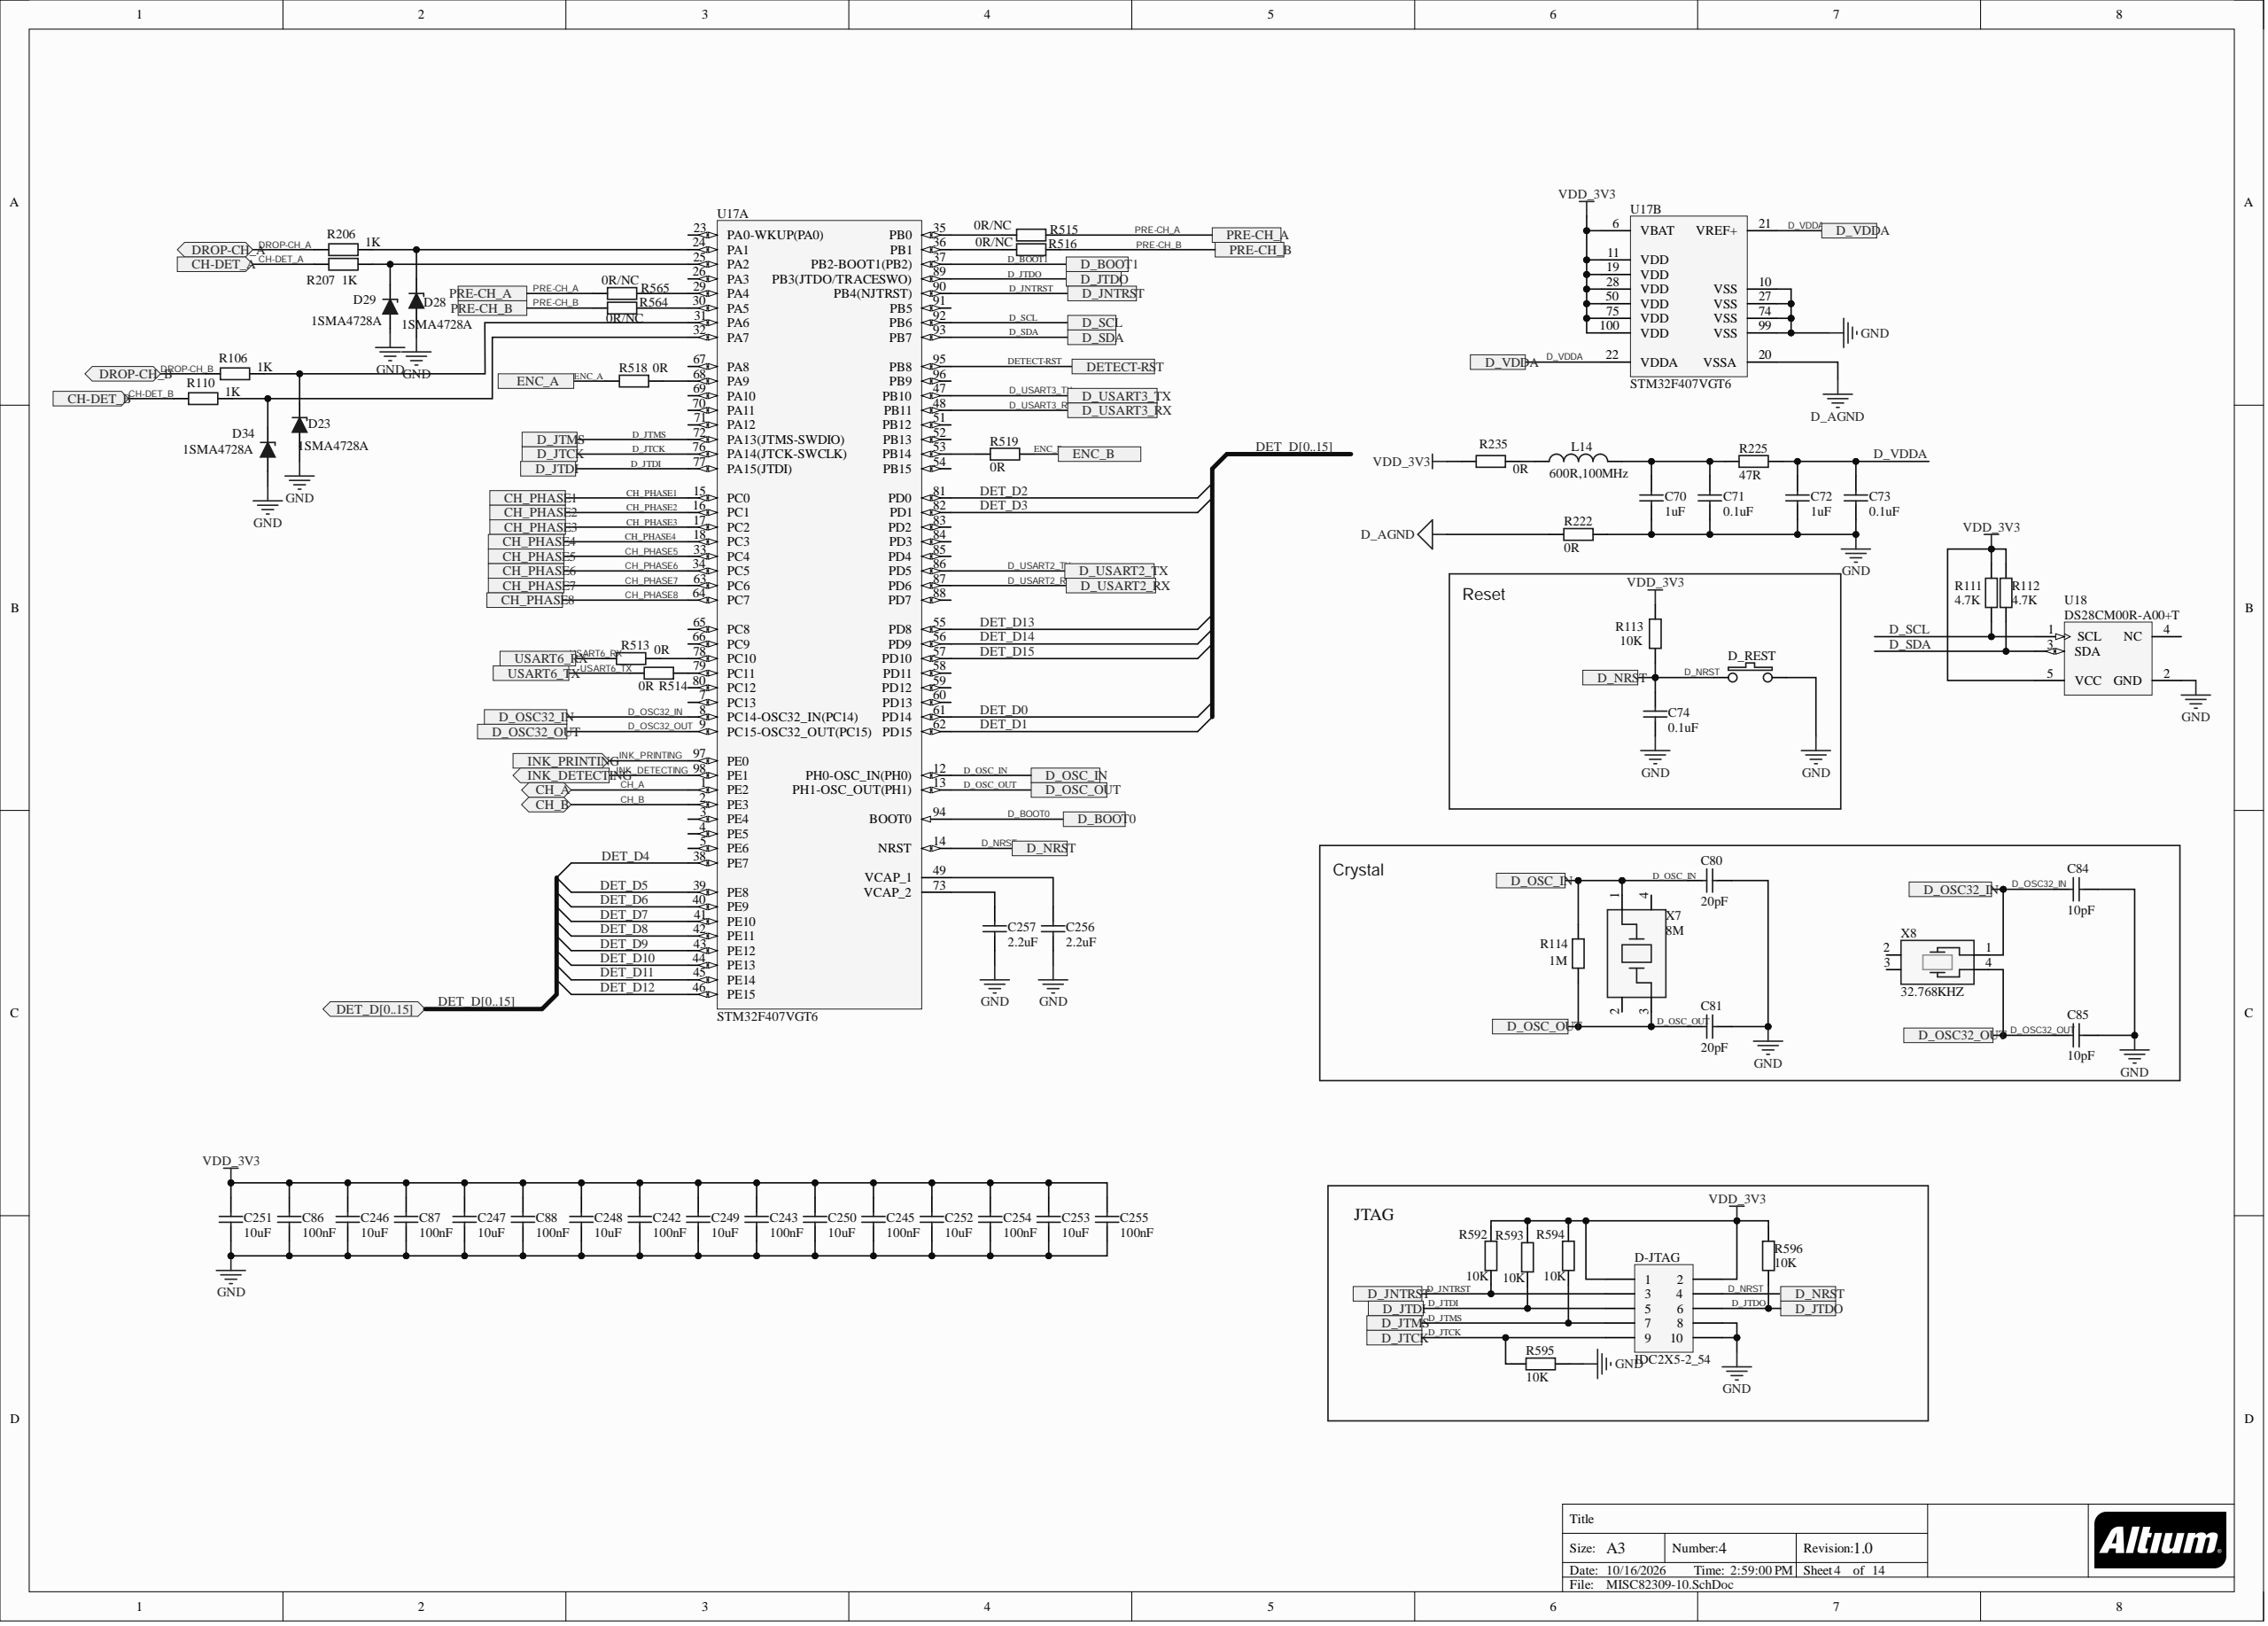Circuit board | Altium Designer | 747 parts | 576 nets | one sheet of the schematic
Parts on this sheet (reference | value | footprint):
C70 | 1uF | CAP_0805
C71 | 0.1uF | CAP_0805
C72 | 1uF | CAP_0805
C73 | 0.1uF | CAP_0805
C74 | 0.1uF | C0603
C80 | 20pF | C0603
C81 | 20pF | C0603
C84 | 10pF | C0603
C85 | 10pF | C0603
C86 | 100nF | C0805
C87 | 100nF | C0805
C88 | 100nF | C0805
C242 | 100nF | C0805
C243 | 100nF | C0805
C245 | 100nF | C0805
C246 | 10uF | C0805
C247 | 10uF | C0805
C248 | 10uF | C0805
C249 | 10uF | C0805
C250 | 10uF | C0805
C251 | 10uF | C0805
C252 | 10uF | C0805
C253 | 10uF | C0805
C254 | 100nF | C0805
C255 | 100nF | C0805
C256 | 2.2uF | CAP_0805
C257 | 2.2uF | CAP_0805
D23 | 1SMA4728A | DO-214AC
D28 | 1SMA4728A | DO-214AC
D29 | 1SMA4728A | DO-214AC
D34 | 1SMA4728A | DO-214AC
D-JTAG | IDC2X5-2_54 | IDC2X5-2_54
D_REST | SW | SW-6X3X2.5
L14 | 600R,100MHz | R0805
R106 | 1K | R1206
R110 | 1K | R1206
R111 | 4.7K | R0603
R112 | 4.7K | R0603
R113 | 10K | R0603
R114 | 1M | R0603
R206 | 1K | R1206
R207 | 1K | R1206
R222 | 0R | R0805
R225 | 47R | R0805
R235 | 0R | R0805
R513 | 0R | RES_0603
R514 | 0R | RES_0603
R515 | 0R/NC | RES_0603
R516 | 0R/NC | RES_0603
R518 | 0R | RES_0603
R519 | 0R | RES_0603
R564 | 0R/NC | RES_0603
R565 | 0R/NC | RES_0603
R592 | 10K | R0603
R593 | 10K | R0603
R594 | 10K | R0603
R595 | 10K | R0603
R596 | 10K | R0603
U17 | STM32F407VGT6 | LQFP100_N
U18 | DS28CM00R-A00+T | U5+1_N
X7 | 8M | SMD5032
X8 | 32.768KHz | Y_XTAL_T7
Nets of these parts (net: part-pin ...):
VDD_3V3: C86-2 C87-2 C88-2 C242-2 C243-2 C245-2 C246-2 C247-2 C248-2 C249-2 C250-2 C251-2 C252-2 C253-2 C254-2 C255-2 D-JTAG-1 D-JTAG-2 R111-1 R112-1 R113-1 R235-1 R592-2 R593-2 R594-2 R596-1 U18-5 U17-6 U17-11 U17-19 U17-28 U17-50 U17-75 U17-100
USART6_TX: R514-2
USART6_RX: R513-2
PRE-CH_B: R516-2 R564-1
PRE-CH_A: R515-2 R565-1
NetR565_2: R565-2 U17-29
NetR564_2: R564-2 U17-30
NetR519_1: R519-1 U17-53
NetR518_1: R518-1 U17-68
NetR516_1: R516-1 U17-36
NetR515_1: R515-1 U17-35
NetR514_1: R514-1 U17-79
NetR513_1: R513-1 U17-78
NetL14_1: L14-1 R235-2
NetD34_2: D34-2 R110-2 U17-32
NetD29_2: D29-2 R207-2 U17-25
NetD28_2: D28-2 R206-2 U17-24
NetD23_2: D23-2 R106-2 U17-31
NetC257_1: C257-1 U17-73
NetC256_1: C256-1 U17-49
NetC70_2: C70-2 C71-2 L14-2 R225-1
INK_PRINTING: U17-97
INK_DETECTING: U17-98
GND: C70-1 C71-1 C72-1 C73-1 C74-1 C80-1 C81-1 C84-1 C85-1 C86-1 C87-1 C88-1 C242-1 C243-1 C245-1 C246-1 C247-1 C248-1 C249-1 C250-1 C251-1 C252-1 C253-1 C254-1 C255-1 C256-2 C257-2 D23-1 D28-1 D29-1 D34-1 D-JTAG-8 D-JTAG-10 D_REST-2 R222-2 R595-1 U18-2 U17-10 U17-27 U17-74 U17-99
ENC_B: R519-2
ENC_A: R518-2
DROP-CH_B: R106-1
DROP-CH_A: R206-1
DETECT-RST: U17-95
DET_D15: U17-57
DET_D14: U17-56
DET_D13: U17-55
DET_D12: U17-46
DET_D11: U17-45
DET_D10: U17-44
DET_D9: U17-43
DET_D8: U17-42
DET_D7: U17-41
DET_D6: U17-40
DET_D5: U17-39
DET_D4: U17-38
DET_D3: U17-82
DET_D2: U17-81
DET_D1: U17-62
DET_D0: U17-61
D_VDDA: C72-2 C73-2 R225-2 U17-21 U17-22
D_USART3_TX: U17-47
D_USART3_RX: U17-48
D_USART2_TX: U17-86
D_USART2_RX: U17-87
D_SDA: R112-2 U18-3 U17-93
D_SCL: R111-2 U18-1 U17-92
D_OSC_OUT: C81-2 R114-2 X7-3 U17-13
D_OSC_IN: C80-2 R114-1 X7-1 U17-12
D_OSC32_OUT: C85-2 X8-4 U17-9
D_OSC32_IN: C84-2 X8-1 U17-8
D_NRST: C74-2 D-JTAG-4 D_REST-1 R113-2 U17-14
D_JTMS: D-JTAG-7 R594-1 U17-72
D_JTDO: D-JTAG-6 R596-2 U17-89
D_JTDI: D-JTAG-5 R593-1 U17-77
D_JTCK: D-JTAG-9 R595-2 U17-76
D_JNTRST: D-JTAG-3 R592-1 U17-90
D_BOOT1: U17-37
D_BOOT0: U17-94
D_AGND: R222-1 U17-20
CH_PHASE8: U17-64
CH_PHASE7: U17-63
CH_PHASE6: U17-34
CH_PHASE5: U17-33
CH_PHASE4: U17-18
CH_PHASE3: U17-17
CH_PHASE2: U17-16
CH_PHASE1: U17-15
CH_B: U17-2
CH_A: U17-1
CH-DET_B: R110-1
CH-DET_A: R207-1